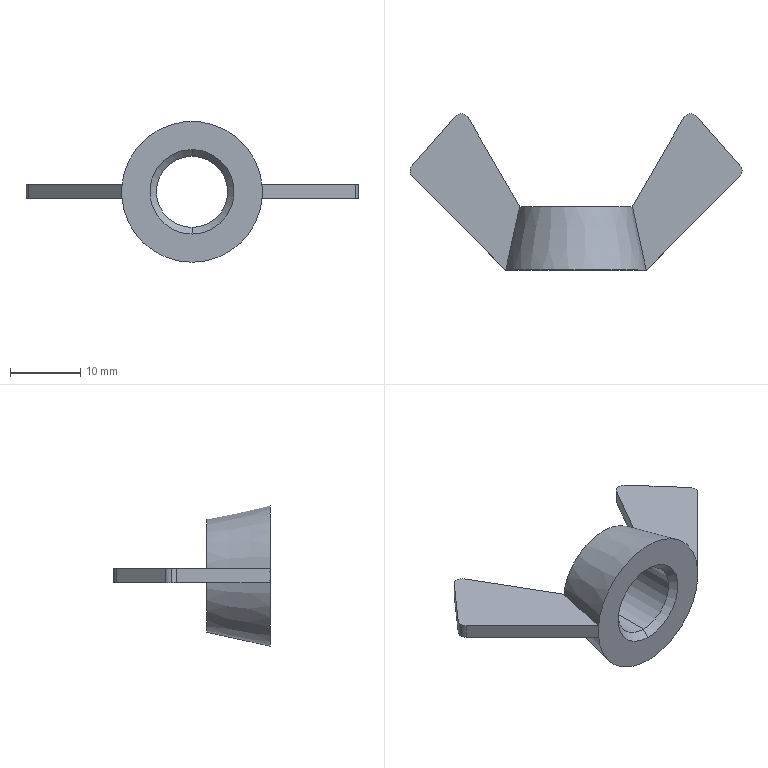Part | SolidWorks | features BaseBody 1 | 1 solid | 32 faces | box 47.146 x 22.189 x 20 mm | volume 2219 mm3 | plane 16 | cone 9 | cylinder 7 | commonest cylinder face diameters 2.3 x5 10.106 x2
STEP:
#1=CARTESIAN_POINT('',(-23.573,9.57,1.));
#2=VERTEX_POINT('',#1);
#3=CARTESIAN_POINT('',(-23.236,8.756,1.));
#4=VERTEX_POINT('',#3);
#5=CARTESIAN_POINT('',(-22.423,9.57,1.));
#6=DIRECTION('',(0.,0.,1.));
#7=DIRECTION('',(1.,0.,0.));
#8=AXIS2_PLACEMENT_3D('',#5,#6,#7);
#9=CIRCLE('',#8,1.15);
#10=EDGE_CURVE('',#2,#4,#9,.T.);
#11=ORIENTED_EDGE('',*,*,#10,.F.);
#12=CARTESIAN_POINT('',(-23.573,9.57,-1.));
#13=VERTEX_POINT('',#12);
#14=CARTESIAN_POINT('',(-23.573,9.57,1.));
#15=DIRECTION('',(0.,0.,-1.));
#16=VECTOR('',#15,1000.);
#17=LINE('',#14,#16);
#18=EDGE_CURVE('',#2,#13,#17,.T.);
#19=ORIENTED_EDGE('',*,*,#18,.T.);
#20=CARTESIAN_POINT('',(-23.236,8.756,-1.));
#21=VERTEX_POINT('',#20);
#22=CARTESIAN_POINT('',(-22.423,9.57,-1.));
#23=DIRECTION('',(0.,0.,1.));
#24=DIRECTION('',(1.,0.,0.));
#25=AXIS2_PLACEMENT_3D('',#22,#23,#24);
#26=CIRCLE('',#25,1.15);
#27=EDGE_CURVE('',#13,#21,#26,.T.);
#28=ORIENTED_EDGE('',*,*,#27,.T.);
#29=CARTESIAN_POINT('',(-23.236,8.756,1.));
#30=DIRECTION('',(0.,0.,-1.));
#31=VECTOR('',#30,1000.);
#32=LINE('',#29,#31);
#33=EDGE_CURVE('',#4,#21,#32,.T.);
#34=ORIENTED_EDGE('',*,*,#33,.F.);
#35=EDGE_LOOP('',(#11,#19,#28,#34));
#36=FACE_OUTER_BOUND('',#35,.T.);
#37=CARTESIAN_POINT('',(-22.423,9.57,1.));
#38=DIRECTION('',(0.,0.,-1.));
#39=DIRECTION('',(-1.,0.,0.));
#40=AXIS2_PLACEMENT_3D('',#37,#38,#39);
#41=CYLINDRICAL_SURFACE('',#40,1.15);
#42=ADVANCED_FACE('',(#36),#41,.T.);
#43=CARTESIAN_POINT('',(0.,3.553,5.053));
#44=VERTEX_POINT('',#43);
#45=CARTESIAN_POINT('',(0.,3.553,-5.053));
#46=VERTEX_POINT('',#45);
#47=CARTESIAN_POINT('',(0.,3.553,0.));
#48=DIRECTION('',(0.,-1.,0.));
#49=DIRECTION('',(0.,0.,-1.));
#50=AXIS2_PLACEMENT_3D('',#47,#48,#49);
#51=CIRCLE('',#50,5.053);
#52=EDGE_CURVE('',#44,#46,#51,.T.);
#53=ORIENTED_EDGE('',*,*,#52,.T.);
#54=CARTESIAN_POINT('',(0.,4.5,-6.));
#55=VERTEX_POINT('',#54);
#56=CARTESIAN_POINT('',(0.,4.5,-6.));
#57=DIRECTION('',(0.,0.7071,-0.7071));
#58=VECTOR('',#57,1000.);
#59=LINE('',#56,#58);
#60=EDGE_CURVE('',#46,#55,#59,.T.);
#61=ORIENTED_EDGE('',*,*,#60,.T.);
#62=CARTESIAN_POINT('',(0.,4.5,6.));
#63=VERTEX_POINT('',#62);
#64=CARTESIAN_POINT('',(0.,4.5,0.));
#65=DIRECTION('',(0.,-1.,0.));
#66=DIRECTION('',(0.,0.,-1.));
#67=AXIS2_PLACEMENT_3D('',#64,#65,#66);
#68=CIRCLE('',#67,6.);
#69=EDGE_CURVE('',#63,#55,#68,.T.);
#70=ORIENTED_EDGE('',*,*,#69,.F.);
#71=CARTESIAN_POINT('',(0.,4.5,6.));
#72=DIRECTION('',(0.,0.7071,0.7071));
#73=VECTOR('',#72,1000.);
#74=LINE('',#71,#73);
#75=EDGE_CURVE('',#44,#63,#74,.T.);
#76=ORIENTED_EDGE('',*,*,#75,.F.);
#77=EDGE_LOOP('',(#53,#61,#70,#76));
#78=FACE_OUTER_BOUND('',#77,.T.);
#79=CARTESIAN_POINT('',(0.,4.5,0.));
#80=DIRECTION('',(0.,1.,0.));
#81=DIRECTION('',(0.,0.,1.));
#82=AXIS2_PLACEMENT_3D('',#79,#80,#81);
#83=CONICAL_SURFACE('',#82,6.,0.7854);
#84=ADVANCED_FACE('',(#78),#83,.F.);
#85=ORIENTED_EDGE('',*,*,#52,.F.);
#86=CARTESIAN_POINT('',(0.,-3.553,5.053));
#87=VERTEX_POINT('',#86);
#88=CARTESIAN_POINT('',(0.,4.5,5.053));
#89=DIRECTION('',(0.,-1.,0.));
#90=VECTOR('',#89,1000.);
#91=LINE('',#88,#90);
#92=EDGE_CURVE('',#44,#87,#91,.T.);
#93=ORIENTED_EDGE('',*,*,#92,.T.);
#94=CARTESIAN_POINT('',(0.,-3.553,-5.053));
#95=VERTEX_POINT('',#94);
#96=CARTESIAN_POINT('',(0.,-3.553,0.));
#97=DIRECTION('',(0.,-1.,0.));
#98=DIRECTION('',(0.,0.,-1.));
#99=AXIS2_PLACEMENT_3D('',#96,#97,#98);
#100=CIRCLE('',#99,5.053);
#101=EDGE_CURVE('',#87,#95,#100,.T.);
#102=ORIENTED_EDGE('',*,*,#101,.T.);
#103=CARTESIAN_POINT('',(0.,4.5,-5.053));
#104=DIRECTION('',(0.,-1.,0.));
#105=VECTOR('',#104,1000.);
#106=LINE('',#103,#105);
#107=EDGE_CURVE('',#46,#95,#106,.T.);
#108=ORIENTED_EDGE('',*,*,#107,.F.);
#109=EDGE_LOOP('',(#85,#93,#102,#108));
#110=FACE_OUTER_BOUND('',#109,.T.);
#111=CARTESIAN_POINT('',(0.,4.5,0.));
#112=DIRECTION('',(0.,-1.,0.));
#113=DIRECTION('',(0.,0.,-1.));
#114=AXIS2_PLACEMENT_3D('',#111,#112,#113);
#115=CYLINDRICAL_SURFACE('',#114,5.053);
#116=ADVANCED_FACE('',(#110),#115,.F.);
#117=ORIENTED_EDGE('',*,*,#101,.F.);
#118=CARTESIAN_POINT('',(0.,-4.5,6.));
#119=VERTEX_POINT('',#118);
#120=CARTESIAN_POINT('',(0.,-3.553,5.053));
#121=DIRECTION('',(0.,-0.7071,0.7071));
#122=VECTOR('',#121,1000.);
#123=LINE('',#120,#122);
#124=EDGE_CURVE('',#87,#119,#123,.T.);
#125=ORIENTED_EDGE('',*,*,#124,.T.);
#126=CARTESIAN_POINT('',(0.,-4.5,-6.));
#127=VERTEX_POINT('',#126);
#128=CARTESIAN_POINT('',(0.,-4.5,0.));
#129=DIRECTION('',(0.,-1.,0.));
#130=DIRECTION('',(0.,0.,-1.));
#131=AXIS2_PLACEMENT_3D('',#128,#129,#130);
#132=CIRCLE('',#131,6.);
#133=EDGE_CURVE('',#119,#127,#132,.T.);
#134=ORIENTED_EDGE('',*,*,#133,.T.);
#135=CARTESIAN_POINT('',(0.,-3.553,-5.053));
#136=DIRECTION('',(0.,-0.7071,-0.7071));
#137=VECTOR('',#136,1000.);
#138=LINE('',#135,#137);
#139=EDGE_CURVE('',#95,#127,#138,.T.);
#140=ORIENTED_EDGE('',*,*,#139,.F.);
#141=EDGE_LOOP('',(#117,#125,#134,#140));
#142=FACE_OUTER_BOUND('',#141,.T.);
#143=CARTESIAN_POINT('',(0.,-3.553,0.));
#144=DIRECTION('',(0.,-1.,0.));
#145=DIRECTION('',(0.,0.,-1.));
#146=AXIS2_PLACEMENT_3D('',#143,#144,#145);
#147=CONICAL_SURFACE('',#146,5.053,0.7854);
#148=ADVANCED_FACE('',(#142),#147,.F.);
#149=CARTESIAN_POINT('',(-8.,4.5,0.));
#150=VERTEX_POINT('',#149);
#151=CARTESIAN_POINT('',(0.,4.5,-8.));
#152=VERTEX_POINT('',#151);
#153=CARTESIAN_POINT('',(0.,4.5,0.));
#154=DIRECTION('',(0.,-1.,0.));
#155=DIRECTION('',(0.,0.,-1.));
#156=AXIS2_PLACEMENT_3D('',#153,#154,#155);
#157=CIRCLE('',#156,8.);
#158=EDGE_CURVE('',#150,#152,#157,.T.);
#159=ORIENTED_EDGE('',*,*,#158,.T.);
#160=CARTESIAN_POINT('',(0.,-4.5,-10.));
#161=VERTEX_POINT('',#160);
#162=CARTESIAN_POINT('',(0.,4.5,-8.));
#163=DIRECTION('',(0.,-0.9762,-0.2169));
#164=VECTOR('',#163,1000.);
#165=LINE('',#162,#164);
#166=EDGE_CURVE('',#152,#161,#165,.T.);
#167=ORIENTED_EDGE('',*,*,#166,.T.);
#168=CARTESIAN_POINT('',(-9.98,-4.5,-0.6321));
#169=VERTEX_POINT('',#168);
#170=CARTESIAN_POINT('',(0.,-4.5,0.));
#171=DIRECTION('',(0.,-1.,0.));
#172=DIRECTION('',(0.,0.,-1.));
#173=AXIS2_PLACEMENT_3D('',#170,#171,#172);
#174=CIRCLE('',#173,10.);
#175=EDGE_CURVE('',#169,#161,#174,.T.);
#176=ORIENTED_EDGE('',*,*,#175,.F.);
#177=CARTESIAN_POINT('',(-8.,4.5,0.));
#178=CARTESIAN_POINT('',(-8.,4.5,-0.01244));
#179=CARTESIAN_POINT('',(-8.003,4.489,-0.02117));
#180=CARTESIAN_POINT('',(-8.007,4.468,-0.03411));
#181=CARTESIAN_POINT('',(-8.009,4.458,-0.03905));
#182=CARTESIAN_POINT('',(-8.017,4.425,-0.0525));
#183=CARTESIAN_POINT('',(-8.022,4.402,-0.0594));
#184=CARTESIAN_POINT('',(-8.037,4.334,-0.07803));
#185=CARTESIAN_POINT('',(-8.047,4.288,-0.08757));
#186=CARTESIAN_POINT('',(-8.077,4.149,-0.1136));
#187=CARTESIAN_POINT('',(-8.098,4.055,-0.1271));
#188=CARTESIAN_POINT('',(-8.16,3.775,-0.1639));
#189=CARTESIAN_POINT('',(-8.201,3.587,-0.1831));
#190=CARTESIAN_POINT('',(-8.325,3.025,-0.236));
#191=CARTESIAN_POINT('',(-8.407,2.649,-0.264));
#192=CARTESIAN_POINT('',(-8.655,1.521,-0.3417));
#193=CARTESIAN_POINT('',(-8.821,0.7688,-0.3839));
#194=CARTESIAN_POINT('',(-9.318,-1.489,-0.5022));
#195=CARTESIAN_POINT('',(-9.649,-2.994,-0.5687));
#196=CARTESIAN_POINT('',(-9.98,-4.5,-0.6321));
#197=B_SPLINE_CURVE_WITH_KNOTS('',3,(#177,#178,#179,#180,#181,#182,#183,#184,#185,#186,#187,#188,#189,#190,#191,#192,#193,#194,#195,#196),.UNSPECIFIED.,.F.,.F.,(4,2,2,2,2,2,2,2,2,4),(0.,0.00003674,0.00007347,0.0001469,0.0002939,0.0005878,0.001176,0.002351,0.004702,0.009405),.UNSPECIFIED.);
#198=EDGE_CURVE('',#150,#169,#197,.T.);
#199=ORIENTED_EDGE('',*,*,#198,.F.);
#200=EDGE_LOOP('',(#159,#167,#176,#199));
#201=FACE_OUTER_BOUND('',#200,.T.);
#202=CARTESIAN_POINT('',(0.,4.5,0.));
#203=DIRECTION('',(0.,-1.,0.));
#204=DIRECTION('',(0.,0.,-1.));
#205=AXIS2_PLACEMENT_3D('',#202,#203,#204);
#206=CONICAL_SURFACE('',#205,8.,0.2187);
#207=ADVANCED_FACE('',(#201),#206,.T.);
#208=CARTESIAN_POINT('',(15.283,17.114,-1.));
#209=VERTEX_POINT('',#208);
#210=CARTESIAN_POINT('',(8.,4.5,-1.));
#211=VERTEX_POINT('',#210);
#212=CARTESIAN_POINT('',(15.283,17.114,-1.));
#213=DIRECTION('',(-0.5,-0.866,0.));
#214=VECTOR('',#213,1000.);
#215=LINE('',#212,#214);
#216=EDGE_CURVE('',#209,#211,#215,.T.);
#217=ORIENTED_EDGE('',*,*,#216,.F.);
#218=CARTESIAN_POINT('',(17.141,17.3,-1.));
#219=VERTEX_POINT('',#218);
#220=CARTESIAN_POINT('',(16.279,16.539,-1.));
#221=DIRECTION('',(0.,0.,1.));
#222=DIRECTION('',(1.,0.,0.));
#223=AXIS2_PLACEMENT_3D('',#220,#221,#222);
#224=CIRCLE('',#223,1.15);
#225=EDGE_CURVE('',#219,#209,#224,.T.);
#226=ORIENTED_EDGE('',*,*,#225,.F.);
#227=CARTESIAN_POINT('',(23.286,10.33,-1.));
#228=VERTEX_POINT('',#227);
#229=CARTESIAN_POINT('',(23.286,10.33,-1.));
#230=DIRECTION('',(-0.6613,0.7501,0.));
#231=VECTOR('',#230,1000.);
#232=LINE('',#229,#231);
#233=EDGE_CURVE('',#228,#219,#232,.T.);
#234=ORIENTED_EDGE('',*,*,#233,.F.);
#235=CARTESIAN_POINT('',(23.236,8.756,-1.));
#236=VERTEX_POINT('',#235);
#237=CARTESIAN_POINT('',(22.423,9.57,-1.));
#238=DIRECTION('',(0.,0.,1.));
#239=DIRECTION('',(1.,0.,0.));
#240=AXIS2_PLACEMENT_3D('',#237,#238,#239);
#241=CIRCLE('',#240,1.15);
#242=EDGE_CURVE('',#236,#228,#241,.T.);
#243=ORIENTED_EDGE('',*,*,#242,.F.);
#244=CARTESIAN_POINT('',(9.98,-4.5,-1.));
#245=VERTEX_POINT('',#244);
#246=CARTESIAN_POINT('',(9.98,-4.5,-1.));
#247=DIRECTION('',(0.7071,0.7071,0.));
#248=VECTOR('',#247,1000.);
#249=LINE('',#246,#248);
#250=EDGE_CURVE('',#245,#236,#249,.T.);
#251=ORIENTED_EDGE('',*,*,#250,.F.);
#252=CARTESIAN_POINT('',(8.,4.5,-1.));
#253=DIRECTION('',(0.2149,-0.9766,0.));
#254=VECTOR('',#253,1000.);
#255=LINE('',#252,#254);
#256=EDGE_CURVE('',#211,#245,#255,.T.);
#257=ORIENTED_EDGE('',*,*,#256,.F.);
#258=EDGE_LOOP('',(#217,#226,#234,#243,#251,#257));
#259=FACE_OUTER_BOUND('',#258,.T.);
#260=CARTESIAN_POINT('',(22.423,9.57,-1.));
#261=DIRECTION('',(0.,0.,1.));
#262=DIRECTION('',(1.,0.,0.));
#263=AXIS2_PLACEMENT_3D('',#260,#261,#262);
#264=PLANE('',#263);
#265=ADVANCED_FACE('',(#259),#264,.F.);
#266=CARTESIAN_POINT('',(15.283,17.114,1.));
#267=VERTEX_POINT('',#266);
#268=CARTESIAN_POINT('',(8.,4.5,1.));
#269=VERTEX_POINT('',#268);
#270=CARTESIAN_POINT('',(15.283,17.114,1.));
#271=DIRECTION('',(-0.5,-0.866,0.));
#272=VECTOR('',#271,1000.);
#273=LINE('',#270,#272);
#274=EDGE_CURVE('',#267,#269,#273,.T.);
#275=ORIENTED_EDGE('',*,*,#274,.T.);
#276=CARTESIAN_POINT('',(9.98,-4.5,1.));
#277=VERTEX_POINT('',#276);
#278=CARTESIAN_POINT('',(8.,4.5,1.));
#279=DIRECTION('',(0.2149,-0.9766,0.));
#280=VECTOR('',#279,1000.);
#281=LINE('',#278,#280);
#282=EDGE_CURVE('',#269,#277,#281,.T.);
#283=ORIENTED_EDGE('',*,*,#282,.T.);
#284=CARTESIAN_POINT('',(23.236,8.756,1.));
#285=VERTEX_POINT('',#284);
#286=CARTESIAN_POINT('',(9.98,-4.5,1.));
#287=DIRECTION('',(0.7071,0.7071,0.));
#288=VECTOR('',#287,1000.);
#289=LINE('',#286,#288);
#290=EDGE_CURVE('',#277,#285,#289,.T.);
#291=ORIENTED_EDGE('',*,*,#290,.T.);
#292=CARTESIAN_POINT('',(23.286,10.33,1.));
#293=VERTEX_POINT('',#292);
#294=CARTESIAN_POINT('',(22.423,9.57,1.));
#295=DIRECTION('',(0.,0.,1.));
#296=DIRECTION('',(1.,0.,0.));
#297=AXIS2_PLACEMENT_3D('',#294,#295,#296);
#298=CIRCLE('',#297,1.15);
#299=EDGE_CURVE('',#285,#293,#298,.T.);
#300=ORIENTED_EDGE('',*,*,#299,.T.);
#301=CARTESIAN_POINT('',(17.141,17.3,1.));
#302=VERTEX_POINT('',#301);
#303=CARTESIAN_POINT('',(23.286,10.33,1.));
#304=DIRECTION('',(-0.6613,0.7501,0.));
#305=VECTOR('',#304,1000.);
#306=LINE('',#303,#305);
#307=EDGE_CURVE('',#293,#302,#306,.T.);
#308=ORIENTED_EDGE('',*,*,#307,.T.);
#309=CARTESIAN_POINT('',(16.279,16.539,1.));
#310=DIRECTION('',(0.,0.,1.));
#311=DIRECTION('',(1.,0.,0.));
#312=AXIS2_PLACEMENT_3D('',#309,#310,#311);
#313=CIRCLE('',#312,1.15);
#314=EDGE_CURVE('',#302,#267,#313,.T.);
#315=ORIENTED_EDGE('',*,*,#314,.T.);
#316=EDGE_LOOP('',(#275,#283,#291,#300,#308,#315));
#317=FACE_OUTER_BOUND('',#316,.T.);
#318=CARTESIAN_POINT('',(22.423,9.57,1.));
#319=DIRECTION('',(0.,0.,1.));
#320=DIRECTION('',(1.,0.,0.));
#321=AXIS2_PLACEMENT_3D('',#318,#319,#320);
#322=PLANE('',#321);
#323=ADVANCED_FACE('',(#317),#322,.T.);
#324=CARTESIAN_POINT('',(17.141,17.3,1.));
#325=DIRECTION('',(0.,0.,-1.));
#326=VECTOR('',#325,1000.);
#327=LINE('',#324,#326);
#328=EDGE_CURVE('',#302,#219,#327,.T.);
#329=ORIENTED_EDGE('',*,*,#328,.T.);
#330=ORIENTED_EDGE('',*,*,#225,.T.);
#331=CARTESIAN_POINT('',(15.283,17.114,1.));
#332=DIRECTION('',(0.,0.,-1.));
#333=VECTOR('',#332,1000.);
#334=LINE('',#331,#333);
#335=EDGE_CURVE('',#267,#209,#334,.T.);
#336=ORIENTED_EDGE('',*,*,#335,.F.);
#337=ORIENTED_EDGE('',*,*,#314,.F.);
#338=EDGE_LOOP('',(#329,#330,#336,#337));
#339=FACE_OUTER_BOUND('',#338,.T.);
#340=CARTESIAN_POINT('',(16.279,16.539,1.));
#341=DIRECTION('',(0.,0.,-1.));
#342=DIRECTION('',(-1.,0.,0.));
#343=AXIS2_PLACEMENT_3D('',#340,#341,#342);
#344=CYLINDRICAL_SURFACE('',#343,1.15);
#345=ADVANCED_FACE('',(#339),#344,.T.);
#346=CARTESIAN_POINT('',(23.286,10.33,1.));
#347=DIRECTION('',(0.,0.,-1.));
#348=VECTOR('',#347,1000.);
#349=LINE('',#346,#348);
#350=EDGE_CURVE('',#293,#228,#349,.T.);
#351=ORIENTED_EDGE('',*,*,#350,.T.);
#352=ORIENTED_EDGE('',*,*,#233,.T.);
#353=ORIENTED_EDGE('',*,*,#328,.F.);
#354=ORIENTED_EDGE('',*,*,#307,.F.);
#355=EDGE_LOOP('',(#351,#352,#353,#354));
#356=FACE_OUTER_BOUND('',#355,.T.);
#357=CARTESIAN_POINT('',(23.286,10.33,1.));
#358=DIRECTION('',(-0.7501,-0.6613,0.));
#359=DIRECTION('',(-0.6613,0.7501,0.));
#360=AXIS2_PLACEMENT_3D('',#357,#358,#359);
#361=PLANE('',#360);
#362=ADVANCED_FACE('',(#356),#361,.F.);
#363=CARTESIAN_POINT('',(23.236,8.756,1.));
#364=DIRECTION('',(0.,0.,-1.));
#365=VECTOR('',#364,1000.);
#366=LINE('',#363,#365);
#367=EDGE_CURVE('',#285,#236,#366,.T.);
#368=ORIENTED_EDGE('',*,*,#367,.T.);
#369=ORIENTED_EDGE('',*,*,#242,.T.);
#370=ORIENTED_EDGE('',*,*,#350,.F.);
#371=ORIENTED_EDGE('',*,*,#299,.F.);
#372=EDGE_LOOP('',(#368,#369,#370,#371));
#373=FACE_OUTER_BOUND('',#372,.T.);
#374=CARTESIAN_POINT('',(22.423,9.57,1.));
#375=DIRECTION('',(0.,0.,-1.));
#376=DIRECTION('',(-1.,0.,0.));
#377=AXIS2_PLACEMENT_3D('',#374,#375,#376);
#378=CYLINDRICAL_SURFACE('',#377,1.15);
#379=ADVANCED_FACE('',(#373),#378,.T.);
#380=ORIENTED_EDGE('',*,*,#335,.T.);
#381=ORIENTED_EDGE('',*,*,#216,.T.);
#382=CARTESIAN_POINT('',(8.,4.5,0.));
#383=VERTEX_POINT('',#382);
#384=CARTESIAN_POINT('',(8.,4.5,1.));
#385=DIRECTION('',(0.,0.,-1.));
#386=VECTOR('',#385,1000.);
#387=LINE('',#384,#386);
#388=EDGE_CURVE('',#383,#211,#387,.T.);
#389=ORIENTED_EDGE('',*,*,#388,.F.);
#390=CARTESIAN_POINT('',(8.,4.5,1.));
#391=DIRECTION('',(0.,0.,-1.));
#392=VECTOR('',#391,1000.);
#393=LINE('',#390,#392);
#394=EDGE_CURVE('',#269,#383,#393,.T.);
#395=ORIENTED_EDGE('',*,*,#394,.F.);
#396=ORIENTED_EDGE('',*,*,#274,.F.);
#397=EDGE_LOOP('',(#380,#381,#389,#395,#396));
#398=FACE_OUTER_BOUND('',#397,.T.);
#399=CARTESIAN_POINT('',(15.283,17.114,1.));
#400=DIRECTION('',(0.866,-0.5,0.));
#401=DIRECTION('',(0.,0.,-1.));
#402=AXIS2_PLACEMENT_3D('',#399,#400,#401);
#403=PLANE('',#402);
#404=ADVANCED_FACE('',(#398),#403,.F.);
#405=ORIENTED_EDGE('',*,*,#394,.T.);
#406=CARTESIAN_POINT('',(9.98,-4.5,0.6321));
#407=VERTEX_POINT('',#406);
#408=CARTESIAN_POINT('',(8.,4.5,0.));
#409=CARTESIAN_POINT('',(8.,4.5,0.01244));
#410=CARTESIAN_POINT('',(8.003,4.489,0.02117));
#411=CARTESIAN_POINT('',(8.007,4.468,0.03411));
#412=CARTESIAN_POINT('',(8.009,4.458,0.03905));
#413=CARTESIAN_POINT('',(8.017,4.425,0.0525));
#414=CARTESIAN_POINT('',(8.022,4.402,0.0594));
#415=CARTESIAN_POINT('',(8.037,4.334,0.07803));
#416=CARTESIAN_POINT('',(8.047,4.288,0.08757));
#417=CARTESIAN_POINT('',(8.077,4.149,0.1136));
#418=CARTESIAN_POINT('',(8.098,4.055,0.1271));
#419=CARTESIAN_POINT('',(8.16,3.775,0.1639));
#420=CARTESIAN_POINT('',(8.201,3.587,0.1831));
#421=CARTESIAN_POINT('',(8.325,3.025,0.236));
#422=CARTESIAN_POINT('',(8.407,2.649,0.264));
#423=CARTESIAN_POINT('',(8.655,1.521,0.3417));
#424=CARTESIAN_POINT('',(8.821,0.7688,0.3839));
#425=CARTESIAN_POINT('',(9.318,-1.489,0.5022));
#426=CARTESIAN_POINT('',(9.649,-2.994,0.5687));
#427=CARTESIAN_POINT('',(9.98,-4.5,0.6321));
#428=B_SPLINE_CURVE_WITH_KNOTS('',3,(#408,#409,#410,#411,#412,#413,#414,#415,#416,#417,#418,#419,#420,#421,#422,#423,#424,#425,#426,#427),.UNSPECIFIED.,.F.,.F.,(4,2,2,2,2,2,2,2,2,4),(0.,0.00003674,0.00007347,0.0001469,0.0002939,0.0005878,0.001176,0.002351,0.004702,0.009405),.UNSPECIFIED.);
#429=EDGE_CURVE('',#383,#407,#428,.T.);
#430=ORIENTED_EDGE('',*,*,#429,.T.);
#431=CARTESIAN_POINT('',(9.98,-4.5,1.));
#432=DIRECTION('',(0.,0.,-1.));
#433=VECTOR('',#432,1000.);
#434=LINE('',#431,#433);
#435=EDGE_CURVE('',#277,#407,#434,.T.);
#436=ORIENTED_EDGE('',*,*,#435,.F.);
#437=ORIENTED_EDGE('',*,*,#282,.F.);
#438=EDGE_LOOP('',(#405,#430,#436,#437));
#439=FACE_OUTER_BOUND('',#438,.T.);
#440=CARTESIAN_POINT('',(8.,4.5,1.));
#441=DIRECTION('',(0.9766,0.2149,0.));
#442=DIRECTION('',(0.,0.,-1.));
#443=AXIS2_PLACEMENT_3D('',#440,#441,#442);
#444=PLANE('',#443);
#445=ADVANCED_FACE('',(#439),#444,.F.);
#446=CARTESIAN_POINT('',(9.98,-4.5,-0.6321));
#447=VERTEX_POINT('',#446);
#448=CARTESIAN_POINT('',(9.98,-4.5,1.));
#449=DIRECTION('',(0.,0.,-1.));
#450=VECTOR('',#449,1000.);
#451=LINE('',#448,#450);
#452=EDGE_CURVE('',#447,#245,#451,.T.);
#453=ORIENTED_EDGE('',*,*,#452,.F.);
#454=CARTESIAN_POINT('',(9.98,-4.5,-0.6321));
#455=CARTESIAN_POINT('',(9.761,-3.505,-0.5902));
#456=CARTESIAN_POINT('',(9.542,-2.51,-0.5466));
#457=CARTESIAN_POINT('',(9.323,-1.515,-0.4994));
#458=CARTESIAN_POINT('',(9.177,-0.8499,-0.4679));
#459=CARTESIAN_POINT('',(9.031,-0.1844,-0.4347));
#460=CARTESIAN_POINT('',(8.884,0.4808,-0.3985));
#461=CARTESIAN_POINT('',(8.786,0.9259,-0.3742));
#462=CARTESIAN_POINT('',(8.688,1.371,-0.3485));
#463=CARTESIAN_POINT('',(8.591,1.816,-0.3202));
#464=CARTESIAN_POINT('',(8.525,2.114,-0.3012));
#465=CARTESIAN_POINT('',(8.46,2.411,-0.281));
#466=CARTESIAN_POINT('',(8.394,2.709,-0.2585));
#467=CARTESIAN_POINT('',(8.35,2.908,-0.2435));
#468=CARTESIAN_POINT('',(8.306,3.107,-0.2274));
#469=CARTESIAN_POINT('',(8.263,3.306,-0.2094));
#470=CARTESIAN_POINT('',(8.233,3.439,-0.1974));
#471=CARTESIAN_POINT('',(8.204,3.572,-0.1845));
#472=CARTESIAN_POINT('',(8.175,3.705,-0.1699));
#473=CARTESIAN_POINT('',(8.155,3.794,-0.1602));
#474=CARTESIAN_POINT('',(8.136,3.884,-0.1497));
#475=CARTESIAN_POINT('',(8.116,3.972,-0.138));
#476=CARTESIAN_POINT('',(8.103,4.032,-0.13));
#477=CARTESIAN_POINT('',(8.09,4.092,-0.1215));
#478=CARTESIAN_POINT('',(8.077,4.151,-0.1119));
#479=CARTESIAN_POINT('',(8.068,4.191,-0.1055));
#480=CARTESIAN_POINT('',(8.059,4.231,-0.0985));
#481=CARTESIAN_POINT('',(8.05,4.27,-0.09062));
#482=CARTESIAN_POINT('',(8.045,4.297,-0.08531));
#483=CARTESIAN_POINT('',(8.039,4.324,-0.07959));
#484=CARTESIAN_POINT('',(8.033,4.35,-0.0731));
#485=CARTESIAN_POINT('',(8.029,4.368,-0.06871));
#486=CARTESIAN_POINT('',(8.025,4.386,-0.06397));
#487=CARTESIAN_POINT('',(8.021,4.404,-0.05859));
#488=CARTESIAN_POINT('',(8.019,4.416,-0.05493));
#489=CARTESIAN_POINT('',(8.016,4.428,-0.05098));
#490=CARTESIAN_POINT('',(8.013,4.439,-0.04648));
#491=CARTESIAN_POINT('',(8.012,4.447,-0.0434));
#492=CARTESIAN_POINT('',(8.01,4.455,-0.04006));
#493=CARTESIAN_POINT('',(8.008,4.463,-0.03626));
#494=CARTESIAN_POINT('',(8.007,4.47,-0.03271));
#495=CARTESIAN_POINT('',(8.005,4.477,-0.02876));
#496=CARTESIAN_POINT('',(8.004,4.484,-0.02393));
#497=CARTESIAN_POINT('',(8.003,4.487,-0.02147));
#498=CARTESIAN_POINT('',(8.002,4.49,-0.01876));
#499=CARTESIAN_POINT('',(8.002,4.493,-0.01566));
#500=CARTESIAN_POINT('',(8.001,4.495,-0.01339));
#501=CARTESIAN_POINT('',(8.001,4.497,-0.01086));
#502=CARTESIAN_POINT('',(8.,4.498,-0.008086));
#503=CARTESIAN_POINT('',(8.,4.499,-0.006137));
#504=CARTESIAN_POINT('',(8.,4.5,-0.004024));
#505=CARTESIAN_POINT('',(8.,4.5,-0.001887));
#506=CARTESIAN_POINT('',(8.,4.5,-0.001261));
#507=CARTESIAN_POINT('',(8.,4.5,-0.0006299));
#508=CARTESIAN_POINT('',(8.,4.5,0.));
#509=B_SPLINE_CURVE_WITH_KNOTS('',3,(#454,#455,#456,#457,#458,#459,#460,#461,#462,#463,#464,#465,#466,#467,#468,#469,#470,#471,#472,#473,#474,#475,#476,#477,#478,#479,#480,#481,#482,#483,#484,#485,#486,#487,#488,#489,#490,#491,#492,#493,#494,#495,#496,#497,#498,#499,#500,#501,#502,#503,#504,#505,#506,#507,#508),.UNSPECIFIED.,.F.,.F.,(4,3,3,3,3,3,3,3,3,3,3,3,3,3,3,3,3,3,4),(0.,0.003059,0.005105,0.006475,0.007391,0.008004,0.008415,0.00869,0.008875,0.008999,0.009083,0.00914,0.009178,0.009204,0.009229,0.009242,0.009251,0.009257,0.009259),.UNSPECIFIED.);
#510=EDGE_CURVE('',#447,#383,#509,.T.);
#511=ORIENTED_EDGE('',*,*,#510,.T.);
#512=ORIENTED_EDGE('',*,*,#388,.T.);
#513=ORIENTED_EDGE('',*,*,#256,.T.);
#514=EDGE_LOOP('',(#453,#511,#512,#513));
#515=FACE_OUTER_BOUND('',#514,.T.);
#516=CARTESIAN_POINT('',(8.,4.5,1.));
#517=DIRECTION('',(0.9766,0.2149,0.));
#518=DIRECTION('',(0.,0.,-1.));
#519=AXIS2_PLACEMENT_3D('',#516,#517,#518);
#520=PLANE('',#519);
#521=ADVANCED_FACE('',(#515),#520,.F.);
#522=ORIENTED_EDGE('',*,*,#435,.T.);
#523=CARTESIAN_POINT('',(9.98,-4.5,0.6321));
#524=CARTESIAN_POINT('',(10.002,-4.478,0.2109));
#525=CARTESIAN_POINT('',(10.002,-4.478,-0.2109));
#526=CARTESIAN_POINT('',(9.98,-4.5,-0.6321));
#527=(BOUNDED_CURVE()B_SPLINE_CURVE(3,(#523,#524,#525,#526),.UNSPECIFIED.,.F.,.F.)B_SPLINE_CURVE_WITH_KNOTS((4,4),(3.091,3.192),.UNSPECIFIED.)CURVE()GEOMETRIC_REPRESENTATION_ITEM()RATIONAL_B_SPLINE_CURVE((1.,0.9992,0.9992,1.))REPRESENTATION_ITEM(''));
#528=EDGE_CURVE('',#407,#447,#527,.T.);
#529=ORIENTED_EDGE('',*,*,#528,.T.);
#530=ORIENTED_EDGE('',*,*,#452,.T.);
#531=ORIENTED_EDGE('',*,*,#250,.T.);
#532=ORIENTED_EDGE('',*,*,#367,.F.);
#533=ORIENTED_EDGE('',*,*,#290,.F.);
#534=EDGE_LOOP('',(#522,#529,#530,#531,#532,#533));
#535=FACE_OUTER_BOUND('',#534,.T.);
#536=CARTESIAN_POINT('',(9.98,-4.5,1.));
#537=DIRECTION('',(-0.7071,0.7071,0.));
#538=DIRECTION('',(0.,0.,1.));
#539=AXIS2_PLACEMENT_3D('',#536,#537,#538);
#540=PLANE('',#539);
#541=ADVANCED_FACE('',(#535),#540,.F.);
#542=CARTESIAN_POINT('',(-23.286,10.33,-1.));
#543=VERTEX_POINT('',#542);
#544=CARTESIAN_POINT('',(-22.423,9.57,-1.));
#545=DIRECTION('',(0.,0.,1.));
#546=DIRECTION('',(1.,0.,0.));
#547=AXIS2_PLACEMENT_3D('',#544,#545,#546);
#548=CIRCLE('',#547,1.15);
#549=EDGE_CURVE('',#543,#13,#548,.T.);
#550=ORIENTED_EDGE('',*,*,#549,.F.);
#551=CARTESIAN_POINT('',(-17.141,17.3,-1.));
#552=VERTEX_POINT('',#551);
#553=CARTESIAN_POINT('',(-17.141,17.3,-1.));
#554=DIRECTION('',(-0.6613,-0.7501,0.));
#555=VECTOR('',#554,1000.);
#556=LINE('',#553,#555);
#557=EDGE_CURVE('',#552,#543,#556,.T.);
#558=ORIENTED_EDGE('',*,*,#557,.F.);
#559=CARTESIAN_POINT('',(-15.283,17.114,-1.));
#560=VERTEX_POINT('',#559);
#561=CARTESIAN_POINT('',(-16.279,16.539,-1.));
#562=DIRECTION('',(0.,0.,1.));
#563=DIRECTION('',(1.,0.,0.));
#564=AXIS2_PLACEMENT_3D('',#561,#562,#563);
#565=CIRCLE('',#564,1.15);
#566=EDGE_CURVE('',#560,#552,#565,.T.);
#567=ORIENTED_EDGE('',*,*,#566,.F.);
#568=CARTESIAN_POINT('',(-8.,4.5,-1.));
#569=VERTEX_POINT('',#568);
#570=CARTESIAN_POINT('',(-8.,4.5,-1.));
#571=DIRECTION('',(-0.5,0.866,0.));
#572=VECTOR('',#571,1000.);
#573=LINE('',#570,#572);
#574=EDGE_CURVE('',#569,#560,#573,.T.);
#575=ORIENTED_EDGE('',*,*,#574,.F.);
#576=CARTESIAN_POINT('',(-9.98,-4.5,-1.));
#577=VERTEX_POINT('',#576);
#578=CARTESIAN_POINT('',(-9.98,-4.5,-1.));
#579=DIRECTION('',(0.2149,0.9766,0.));
#580=VECTOR('',#579,1000.);
#581=LINE('',#578,#580);
#582=EDGE_CURVE('',#577,#569,#581,.T.);
#583=ORIENTED_EDGE('',*,*,#582,.F.);
#584=CARTESIAN_POINT('',(-23.236,8.756,-1.));
#585=DIRECTION('',(0.7071,-0.7071,0.));
#586=VECTOR('',#585,1000.);
#587=LINE('',#584,#586);
#588=EDGE_CURVE('',#21,#577,#587,.T.);
#589=ORIENTED_EDGE('',*,*,#588,.F.);
#590=ORIENTED_EDGE('',*,*,#27,.F.);
#591=EDGE_LOOP('',(#550,#558,#567,#575,#583,#589,#590));
#592=FACE_OUTER_BOUND('',#591,.T.);
#593=CARTESIAN_POINT('',(-22.423,9.57,-1.));
#594=DIRECTION('',(0.,0.,1.));
#595=DIRECTION('',(1.,0.,0.));
#596=AXIS2_PLACEMENT_3D('',#593,#594,#595);
#597=PLANE('',#596);
#598=ADVANCED_FACE('',(#592),#597,.F.);
#599=CARTESIAN_POINT('',(-17.141,17.3,1.));
#600=VERTEX_POINT('',#599);
#601=CARTESIAN_POINT('',(-23.286,10.33,1.));
#602=VERTEX_POINT('',#601);
#603=CARTESIAN_POINT('',(-17.141,17.3,1.));
#604=DIRECTION('',(-0.6613,-0.7501,0.));
#605=VECTOR('',#604,1000.);
#606=LINE('',#603,#605);
#607=EDGE_CURVE('',#600,#602,#606,.T.);
#608=ORIENTED_EDGE('',*,*,#607,.T.);
#609=CARTESIAN_POINT('',(-22.423,9.57,1.));
#610=DIRECTION('',(0.,0.,1.));
#611=DIRECTION('',(1.,0.,0.));
#612=AXIS2_PLACEMENT_3D('',#609,#610,#611);
#613=CIRCLE('',#612,1.15);
#614=EDGE_CURVE('',#602,#2,#613,.T.);
#615=ORIENTED_EDGE('',*,*,#614,.T.);
#616=ORIENTED_EDGE('',*,*,#10,.T.);
#617=CARTESIAN_POINT('',(-9.98,-4.5,1.));
#618=VERTEX_POINT('',#617);
#619=CARTESIAN_POINT('',(-23.236,8.756,1.));
#620=DIRECTION('',(0.7071,-0.7071,0.));
#621=VECTOR('',#620,1000.);
#622=LINE('',#619,#621);
#623=EDGE_CURVE('',#4,#618,#622,.T.);
#624=ORIENTED_EDGE('',*,*,#623,.T.);
#625=CARTESIAN_POINT('',(-8.,4.5,1.));
#626=VERTEX_POINT('',#625);
#627=CARTESIAN_POINT('',(-9.98,-4.5,1.));
#628=DIRECTION('',(0.2149,0.9766,0.));
#629=VECTOR('',#628,1000.);
#630=LINE('',#627,#629);
#631=EDGE_CURVE('',#618,#626,#630,.T.);
#632=ORIENTED_EDGE('',*,*,#631,.T.);
#633=CARTESIAN_POINT('',(-15.283,17.114,1.));
#634=VERTEX_POINT('',#633);
#635=CARTESIAN_POINT('',(-8.,4.5,1.));
#636=DIRECTION('',(-0.5,0.866,0.));
#637=VECTOR('',#636,1000.);
#638=LINE('',#635,#637);
#639=EDGE_CURVE('',#626,#634,#638,.T.);
#640=ORIENTED_EDGE('',*,*,#639,.T.);
#641=CARTESIAN_POINT('',(-16.279,16.539,1.));
#642=DIRECTION('',(0.,0.,1.));
#643=DIRECTION('',(1.,0.,0.));
#644=AXIS2_PLACEMENT_3D('',#641,#642,#643);
#645=CIRCLE('',#644,1.15);
#646=EDGE_CURVE('',#634,#600,#645,.T.);
#647=ORIENTED_EDGE('',*,*,#646,.T.);
#648=EDGE_LOOP('',(#608,#615,#616,#624,#632,#640,#647));
#649=FACE_OUTER_BOUND('',#648,.T.);
#650=CARTESIAN_POINT('',(-22.423,9.57,1.));
#651=DIRECTION('',(0.,0.,1.));
#652=DIRECTION('',(1.,0.,0.));
#653=AXIS2_PLACEMENT_3D('',#650,#651,#652);
#654=PLANE('',#653);
#655=ADVANCED_FACE('',(#649),#654,.T.);
#656=CARTESIAN_POINT('',(-17.141,17.3,1.));
#657=DIRECTION('',(0.,0.,-1.));
#658=VECTOR('',#657,1000.);
#659=LINE('',#656,#658);
#660=EDGE_CURVE('',#600,#552,#659,.T.);
#661=ORIENTED_EDGE('',*,*,#660,.T.);
#662=ORIENTED_EDGE('',*,*,#557,.T.);
#663=CARTESIAN_POINT('',(-23.286,10.33,1.));
#664=DIRECTION('',(0.,0.,-1.));
#665=VECTOR('',#664,1000.);
#666=LINE('',#663,#665);
#667=EDGE_CURVE('',#602,#543,#666,.T.);
#668=ORIENTED_EDGE('',*,*,#667,.F.);
#669=ORIENTED_EDGE('',*,*,#607,.F.);
#670=EDGE_LOOP('',(#661,#662,#668,#669));
#671=FACE_OUTER_BOUND('',#670,.T.);
#672=CARTESIAN_POINT('',(-17.141,17.3,1.));
#673=DIRECTION('',(0.7501,-0.6613,0.));
#674=DIRECTION('',(0.,0.,-1.));
#675=AXIS2_PLACEMENT_3D('',#672,#673,#674);
#676=PLANE('',#675);
#677=ADVANCED_FACE('',(#671),#676,.F.);
#678=CARTESIAN_POINT('',(-15.283,17.114,1.));
#679=DIRECTION('',(0.,0.,-1.));
#680=VECTOR('',#679,1000.);
#681=LINE('',#678,#680);
#682=EDGE_CURVE('',#634,#560,#681,.T.);
#683=ORIENTED_EDGE('',*,*,#682,.T.);
#684=ORIENTED_EDGE('',*,*,#566,.T.);
#685=ORIENTED_EDGE('',*,*,#660,.F.);
#686=ORIENTED_EDGE('',*,*,#646,.F.);
#687=EDGE_LOOP('',(#683,#684,#685,#686));
#688=FACE_OUTER_BOUND('',#687,.T.);
#689=CARTESIAN_POINT('',(-16.279,16.539,1.));
#690=DIRECTION('',(0.,0.,-1.));
#691=DIRECTION('',(-1.,0.,0.));
#692=AXIS2_PLACEMENT_3D('',#689,#690,#691);
#693=CYLINDRICAL_SURFACE('',#692,1.15);
#694=ADVANCED_FACE('',(#688),#693,.T.);
#695=CARTESIAN_POINT('',(-8.,4.5,1.));
#696=DIRECTION('',(0.,0.,-1.));
#697=VECTOR('',#696,1000.);
#698=LINE('',#695,#697);
#699=EDGE_CURVE('',#626,#150,#698,.T.);
#700=ORIENTED_EDGE('',*,*,#699,.T.);
#701=CARTESIAN_POINT('',(-8.,4.5,1.));
#702=DIRECTION('',(0.,0.,-1.));
#703=VECTOR('',#702,1000.);
#704=LINE('',#701,#703);
#705=EDGE_CURVE('',#150,#569,#704,.T.);
#706=ORIENTED_EDGE('',*,*,#705,.T.);
#707=ORIENTED_EDGE('',*,*,#574,.T.);
#708=ORIENTED_EDGE('',*,*,#682,.F.);
#709=ORIENTED_EDGE('',*,*,#639,.F.);
#710=EDGE_LOOP('',(#700,#706,#707,#708,#709));
#711=FACE_OUTER_BOUND('',#710,.T.);
#712=CARTESIAN_POINT('',(-8.,4.5,1.));
#713=DIRECTION('',(-0.866,-0.5,0.));
#714=DIRECTION('',(-0.5,0.866,0.));
#715=AXIS2_PLACEMENT_3D('',#712,#713,#714);
#716=PLANE('',#715);
#717=ADVANCED_FACE('',(#711),#716,.F.);
#718=ORIENTED_EDGE('',*,*,#705,.F.);
#719=ORIENTED_EDGE('',*,*,#198,.T.);
#720=CARTESIAN_POINT('',(-9.98,-4.5,1.));
#721=DIRECTION('',(0.,0.,-1.));
#722=VECTOR('',#721,1000.);
#723=LINE('',#720,#722);
#724=EDGE_CURVE('',#169,#577,#723,.T.);
#725=ORIENTED_EDGE('',*,*,#724,.T.);
#726=ORIENTED_EDGE('',*,*,#582,.T.);
#727=EDGE_LOOP('',(#718,#719,#725,#726));
#728=FACE_OUTER_BOUND('',#727,.T.);
#729=CARTESIAN_POINT('',(-9.98,-4.5,1.));
#730=DIRECTION('',(-0.9766,0.2149,0.));
#731=DIRECTION('',(0.,0.,1.));
#732=AXIS2_PLACEMENT_3D('',#729,#730,#731);
#733=PLANE('',#732);
#734=ADVANCED_FACE('',(#728),#733,.F.);
#735=CARTESIAN_POINT('',(-9.98,-4.5,0.6321));
#736=VERTEX_POINT('',#735);
#737=CARTESIAN_POINT('',(-9.98,-4.5,1.));
#738=DIRECTION('',(0.,0.,-1.));
#739=VECTOR('',#738,1000.);
#740=LINE('',#737,#739);
#741=EDGE_CURVE('',#618,#736,#740,.T.);
#742=ORIENTED_EDGE('',*,*,#741,.T.);
#743=CARTESIAN_POINT('',(-9.98,-4.5,0.6321));
#744=CARTESIAN_POINT('',(-9.761,-3.505,0.5902));
#745=CARTESIAN_POINT('',(-9.542,-2.51,0.5466));
#746=CARTESIAN_POINT('',(-9.323,-1.515,0.4994));
#747=CARTESIAN_POINT('',(-9.177,-0.8499,0.4679));
#748=CARTESIAN_POINT('',(-9.031,-0.1844,0.4347));
#749=CARTESIAN_POINT('',(-8.884,0.4808,0.3985));
#750=CARTESIAN_POINT('',(-8.786,0.9259,0.3742));
#751=CARTESIAN_POINT('',(-8.688,1.371,0.3485));
#752=CARTESIAN_POINT('',(-8.591,1.816,0.3202));
#753=CARTESIAN_POINT('',(-8.525,2.114,0.3012));
#754=CARTESIAN_POINT('',(-8.46,2.411,0.281));
#755=CARTESIAN_POINT('',(-8.394,2.709,0.2585));
#756=CARTESIAN_POINT('',(-8.35,2.908,0.2435));
#757=CARTESIAN_POINT('',(-8.306,3.107,0.2274));
#758=CARTESIAN_POINT('',(-8.263,3.306,0.2094));
#759=CARTESIAN_POINT('',(-8.233,3.439,0.1974));
#760=CARTESIAN_POINT('',(-8.204,3.572,0.1845));
#761=CARTESIAN_POINT('',(-8.175,3.705,0.1699));
#762=CARTESIAN_POINT('',(-8.155,3.794,0.1602));
#763=CARTESIAN_POINT('',(-8.136,3.884,0.1497));
#764=CARTESIAN_POINT('',(-8.116,3.972,0.138));
#765=CARTESIAN_POINT('',(-8.103,4.032,0.13));
#766=CARTESIAN_POINT('',(-8.09,4.092,0.1215));
#767=CARTESIAN_POINT('',(-8.077,4.151,0.1119));
#768=CARTESIAN_POINT('',(-8.068,4.191,0.1055));
#769=CARTESIAN_POINT('',(-8.059,4.231,0.0985));
#770=CARTESIAN_POINT('',(-8.05,4.27,0.09062));
#771=CARTESIAN_POINT('',(-8.045,4.297,0.08531));
#772=CARTESIAN_POINT('',(-8.039,4.324,0.07959));
#773=CARTESIAN_POINT('',(-8.033,4.35,0.0731));
#774=CARTESIAN_POINT('',(-8.029,4.368,0.06871));
#775=CARTESIAN_POINT('',(-8.025,4.386,0.06397));
#776=CARTESIAN_POINT('',(-8.021,4.404,0.05859));
#777=CARTESIAN_POINT('',(-8.019,4.416,0.05493));
#778=CARTESIAN_POINT('',(-8.016,4.428,0.05098));
#779=CARTESIAN_POINT('',(-8.013,4.439,0.04648));
#780=CARTESIAN_POINT('',(-8.012,4.447,0.0434));
#781=CARTESIAN_POINT('',(-8.01,4.455,0.04006));
#782=CARTESIAN_POINT('',(-8.008,4.463,0.03626));
#783=CARTESIAN_POINT('',(-8.007,4.47,0.03271));
#784=CARTESIAN_POINT('',(-8.005,4.477,0.02876));
#785=CARTESIAN_POINT('',(-8.004,4.484,0.02393));
#786=CARTESIAN_POINT('',(-8.003,4.487,0.02147));
#787=CARTESIAN_POINT('',(-8.002,4.49,0.01876));
#788=CARTESIAN_POINT('',(-8.002,4.493,0.01566));
#789=CARTESIAN_POINT('',(-8.001,4.495,0.01339));
#790=CARTESIAN_POINT('',(-8.001,4.497,0.01086));
#791=CARTESIAN_POINT('',(-8.,4.498,0.008086));
#792=CARTESIAN_POINT('',(-8.,4.499,0.006137));
#793=CARTESIAN_POINT('',(-8.,4.5,0.004024));
#794=CARTESIAN_POINT('',(-8.,4.5,0.001887));
#795=CARTESIAN_POINT('',(-8.,4.5,0.001261));
#796=CARTESIAN_POINT('',(-8.,4.5,0.0006299));
#797=CARTESIAN_POINT('',(-8.,4.5,0.));
#798=B_SPLINE_CURVE_WITH_KNOTS('',3,(#743,#744,#745,#746,#747,#748,#749,#750,#751,#752,#753,#754,#755,#756,#757,#758,#759,#760,#761,#762,#763,#764,#765,#766,#767,#768,#769,#770,#771,#772,#773,#774,#775,#776,#777,#778,#779,#780,#781,#782,#783,#784,#785,#786,#787,#788,#789,#790,#791,#792,#793,#794,#795,#796,#797),.UNSPECIFIED.,.F.,.F.,(4,3,3,3,3,3,3,3,3,3,3,3,3,3,3,3,3,3,4),(0.,0.003059,0.005105,0.006475,0.007391,0.008004,0.008415,0.00869,0.008875,0.008999,0.009083,0.00914,0.009178,0.009204,0.009229,0.009242,0.009251,0.009257,0.009259),.UNSPECIFIED.);
#799=EDGE_CURVE('',#736,#150,#798,.T.);
#800=ORIENTED_EDGE('',*,*,#799,.T.);
#801=ORIENTED_EDGE('',*,*,#699,.F.);
#802=ORIENTED_EDGE('',*,*,#631,.F.);
#803=EDGE_LOOP('',(#742,#800,#801,#802));
#804=FACE_OUTER_BOUND('',#803,.T.);
#805=CARTESIAN_POINT('',(-9.98,-4.5,1.));
#806=DIRECTION('',(-0.9766,0.2149,0.));
#807=DIRECTION('',(0.,0.,1.));
#808=AXIS2_PLACEMENT_3D('',#805,#806,#807);
#809=PLANE('',#808);
#810=ADVANCED_FACE('',(#804),#809,.F.);
#811=ORIENTED_EDGE('',*,*,#724,.F.);
#812=CARTESIAN_POINT('',(-9.98,-4.5,-0.6321));
#813=CARTESIAN_POINT('',(-10.002,-4.478,-0.2109));
#814=CARTESIAN_POINT('',(-10.002,-4.478,0.2109));
#815=CARTESIAN_POINT('',(-9.98,-4.5,0.6321));
#816=(BOUNDED_CURVE()B_SPLINE_CURVE(3,(#812,#813,#814,#815),.UNSPECIFIED.,.F.,.F.)B_SPLINE_CURVE_WITH_KNOTS((4,4),(3.091,3.192),.UNSPECIFIED.)CURVE()GEOMETRIC_REPRESENTATION_ITEM()RATIONAL_B_SPLINE_CURVE((1.,0.9992,0.9992,1.))REPRESENTATION_ITEM(''));
#817=EDGE_CURVE('',#169,#736,#816,.T.);
#818=ORIENTED_EDGE('',*,*,#817,.T.);
#819=ORIENTED_EDGE('',*,*,#741,.F.);
#820=ORIENTED_EDGE('',*,*,#623,.F.);
#821=ORIENTED_EDGE('',*,*,#33,.T.);
#822=ORIENTED_EDGE('',*,*,#588,.T.);
#823=EDGE_LOOP('',(#811,#818,#819,#820,#821,#822));
#824=FACE_OUTER_BOUND('',#823,.T.);
#825=CARTESIAN_POINT('',(-23.236,8.756,1.));
#826=DIRECTION('',(0.7071,0.7071,0.));
#827=DIRECTION('',(0.,0.,-1.));
#828=AXIS2_PLACEMENT_3D('',#825,#826,#827);
#829=PLANE('',#828);
#830=ADVANCED_FACE('',(#824),#829,.F.);
#831=ORIENTED_EDGE('',*,*,#69,.T.);
#832=CARTESIAN_POINT('',(0.,4.5,0.));
#833=DIRECTION('',(0.,-1.,0.));
#834=DIRECTION('',(0.,0.,-1.));
#835=AXIS2_PLACEMENT_3D('',#832,#833,#834);
#836=CIRCLE('',#835,6.);
#837=EDGE_CURVE('',#55,#63,#836,.T.);
#838=ORIENTED_EDGE('',*,*,#837,.T.);
#839=EDGE_LOOP('',(#831,#838));
#840=FACE_BOUND('',#839,.T.);
#841=ORIENTED_EDGE('',*,*,#158,.F.);
#842=CARTESIAN_POINT('',(0.,4.5,0.));
#843=DIRECTION('',(0.,-1.,0.));
#844=DIRECTION('',(0.,0.,-1.));
#845=AXIS2_PLACEMENT_3D('',#842,#843,#844);
#846=CIRCLE('',#845,8.);
#847=EDGE_CURVE('',#383,#150,#846,.T.);
#848=ORIENTED_EDGE('',*,*,#847,.F.);
#849=CARTESIAN_POINT('',(0.,4.5,0.));
#850=DIRECTION('',(0.,-1.,0.));
#851=DIRECTION('',(0.,0.,-1.));
#852=AXIS2_PLACEMENT_3D('',#849,#850,#851);
#853=CIRCLE('',#852,8.);
#854=EDGE_CURVE('',#152,#383,#853,.T.);
#855=ORIENTED_EDGE('',*,*,#854,.F.);
#856=EDGE_LOOP('',(#841,#848,#855));
#857=FACE_OUTER_BOUND('',#856,.T.);
#858=CARTESIAN_POINT('',(-8.,4.5,0.));
#859=DIRECTION('',(0.,-1.,0.));
#860=DIRECTION('',(0.,0.,-1.));
#861=AXIS2_PLACEMENT_3D('',#858,#859,#860);
#862=PLANE('',#861);
#863=ADVANCED_FACE('',(#840,#857),#862,.F.);
#864=CARTESIAN_POINT('',(0.,-4.5,0.));
#865=DIRECTION('',(0.,-1.,0.));
#866=DIRECTION('',(0.,0.,-1.));
#867=AXIS2_PLACEMENT_3D('',#864,#865,#866);
#868=CIRCLE('',#867,6.);
#869=EDGE_CURVE('',#127,#119,#868,.T.);
#870=ORIENTED_EDGE('',*,*,#869,.F.);
#871=ORIENTED_EDGE('',*,*,#133,.F.);
#872=EDGE_LOOP('',(#870,#871));
#873=FACE_BOUND('',#872,.T.);
#874=ORIENTED_EDGE('',*,*,#175,.T.);
#875=CARTESIAN_POINT('',(0.,-4.5,0.));
#876=DIRECTION('',(0.,-1.,0.));
#877=DIRECTION('',(0.,0.,-1.));
#878=AXIS2_PLACEMENT_3D('',#875,#876,#877);
#879=CIRCLE('',#878,10.);
#880=EDGE_CURVE('',#161,#447,#879,.T.);
#881=ORIENTED_EDGE('',*,*,#880,.T.);
#882=CARTESIAN_POINT('',(0.,-4.5,0.));
#883=DIRECTION('',(0.,-1.,0.));
#884=DIRECTION('',(0.,0.,-1.));
#885=AXIS2_PLACEMENT_3D('',#882,#883,#884);
#886=CIRCLE('',#885,10.);
#887=EDGE_CURVE('',#447,#407,#886,.T.);
#888=ORIENTED_EDGE('',*,*,#887,.T.);
#889=CARTESIAN_POINT('',(0.,-4.5,0.));
#890=DIRECTION('',(0.,-1.,0.));
#891=DIRECTION('',(0.,0.,-1.));
#892=AXIS2_PLACEMENT_3D('',#889,#890,#891);
#893=CIRCLE('',#892,10.);
#894=EDGE_CURVE('',#407,#736,#893,.T.);
#895=ORIENTED_EDGE('',*,*,#894,.T.);
#896=CARTESIAN_POINT('',(0.,-4.5,0.));
#897=DIRECTION('',(0.,-1.,0.));
#898=DIRECTION('',(0.,0.,-1.));
#899=AXIS2_PLACEMENT_3D('',#896,#897,#898);
#900=CIRCLE('',#899,10.);
#901=EDGE_CURVE('',#736,#169,#900,.T.);
#902=ORIENTED_EDGE('',*,*,#901,.T.);
#903=EDGE_LOOP('',(#874,#881,#888,#895,#902));
#904=FACE_OUTER_BOUND('',#903,.T.);
#905=CARTESIAN_POINT('',(0.,-4.5,0.));
#906=DIRECTION('',(0.,1.,0.));
#907=DIRECTION('',(1.,0.,0.));
#908=AXIS2_PLACEMENT_3D('',#905,#906,#907);
#909=PLANE('',#908);
#910=ADVANCED_FACE('',(#873,#904),#909,.F.);
#911=ORIENTED_EDGE('',*,*,#817,.F.);
#912=ORIENTED_EDGE('',*,*,#901,.F.);
#913=EDGE_LOOP('',(#911,#912));
#914=FACE_OUTER_BOUND('',#913,.T.);
#915=CARTESIAN_POINT('',(0.,4.5,0.));
#916=DIRECTION('',(0.,-1.,0.));
#917=DIRECTION('',(0.,0.,-1.));
#918=AXIS2_PLACEMENT_3D('',#915,#916,#917);
#919=CONICAL_SURFACE('',#918,8.,0.2187);
#920=ADVANCED_FACE('',(#914),#919,.T.);
#921=ORIENTED_EDGE('',*,*,#528,.F.);
#922=ORIENTED_EDGE('',*,*,#887,.F.);
#923=EDGE_LOOP('',(#921,#922));
#924=FACE_OUTER_BOUND('',#923,.T.);
#925=CARTESIAN_POINT('',(0.,4.5,0.));
#926=DIRECTION('',(0.,-1.,0.));
#927=DIRECTION('',(0.,0.,-1.));
#928=AXIS2_PLACEMENT_3D('',#925,#926,#927);
#929=CONICAL_SURFACE('',#928,8.,0.2187);
#930=ADVANCED_FACE('',(#924),#929,.T.);
#931=ORIENTED_EDGE('',*,*,#429,.F.);
#932=ORIENTED_EDGE('',*,*,#847,.T.);
#933=ORIENTED_EDGE('',*,*,#799,.F.);
#934=ORIENTED_EDGE('',*,*,#894,.F.);
#935=EDGE_LOOP('',(#931,#932,#933,#934));
#936=FACE_OUTER_BOUND('',#935,.T.);
#937=CARTESIAN_POINT('',(0.,4.5,0.));
#938=DIRECTION('',(0.,-1.,0.));
#939=DIRECTION('',(0.,0.,-1.));
#940=AXIS2_PLACEMENT_3D('',#937,#938,#939);
#941=CONICAL_SURFACE('',#940,8.,0.2187);
#942=ADVANCED_FACE('',(#936),#941,.T.);
#943=ORIENTED_EDGE('',*,*,#166,.F.);
#944=ORIENTED_EDGE('',*,*,#854,.T.);
#945=ORIENTED_EDGE('',*,*,#510,.F.);
#946=ORIENTED_EDGE('',*,*,#880,.F.);
#947=EDGE_LOOP('',(#943,#944,#945,#946));
#948=FACE_OUTER_BOUND('',#947,.T.);
#949=CARTESIAN_POINT('',(0.,4.5,0.));
#950=DIRECTION('',(0.,-1.,0.));
#951=DIRECTION('',(0.,0.,-1.));
#952=AXIS2_PLACEMENT_3D('',#949,#950,#951);
#953=CONICAL_SURFACE('',#952,8.,0.2187);
#954=ADVANCED_FACE('',(#948),#953,.T.);
#955=ORIENTED_EDGE('',*,*,#124,.F.);
#956=CARTESIAN_POINT('',(0.,-3.553,0.));
#957=DIRECTION('',(0.,-1.,0.));
#958=DIRECTION('',(0.,0.,-1.));
#959=AXIS2_PLACEMENT_3D('',#956,#957,#958);
#960=CIRCLE('',#959,5.053);
#961=EDGE_CURVE('',#95,#87,#960,.T.);
#962=ORIENTED_EDGE('',*,*,#961,.F.);
#963=ORIENTED_EDGE('',*,*,#139,.T.);
#964=ORIENTED_EDGE('',*,*,#869,.T.);
#965=EDGE_LOOP('',(#955,#962,#963,#964));
#966=FACE_OUTER_BOUND('',#965,.T.);
#967=CARTESIAN_POINT('',(0.,-3.553,0.));
#968=DIRECTION('',(0.,-1.,0.));
#969=DIRECTION('',(0.,0.,-1.));
#970=AXIS2_PLACEMENT_3D('',#967,#968,#969);
#971=CONICAL_SURFACE('',#970,5.053,0.7854);
#972=ADVANCED_FACE('',(#966),#971,.F.);
#973=ORIENTED_EDGE('',*,*,#92,.F.);
#974=CARTESIAN_POINT('',(0.,3.553,0.));
#975=DIRECTION('',(0.,-1.,0.));
#976=DIRECTION('',(0.,0.,-1.));
#977=AXIS2_PLACEMENT_3D('',#974,#975,#976);
#978=CIRCLE('',#977,5.053);
#979=EDGE_CURVE('',#46,#44,#978,.T.);
#980=ORIENTED_EDGE('',*,*,#979,.F.);
#981=ORIENTED_EDGE('',*,*,#107,.T.);
#982=ORIENTED_EDGE('',*,*,#961,.T.);
#983=EDGE_LOOP('',(#973,#980,#981,#982));
#984=FACE_OUTER_BOUND('',#983,.T.);
#985=CARTESIAN_POINT('',(0.,4.5,0.));
#986=DIRECTION('',(0.,-1.,0.));
#987=DIRECTION('',(0.,0.,-1.));
#988=AXIS2_PLACEMENT_3D('',#985,#986,#987);
#989=CYLINDRICAL_SURFACE('',#988,5.053);
#990=ADVANCED_FACE('',(#984),#989,.F.);
#991=ORIENTED_EDGE('',*,*,#60,.F.);
#992=ORIENTED_EDGE('',*,*,#979,.T.);
#993=ORIENTED_EDGE('',*,*,#75,.T.);
#994=ORIENTED_EDGE('',*,*,#837,.F.);
#995=EDGE_LOOP('',(#991,#992,#993,#994));
#996=FACE_OUTER_BOUND('',#995,.T.);
#997=CARTESIAN_POINT('',(0.,4.5,0.));
#998=DIRECTION('',(0.,1.,0.));
#999=DIRECTION('',(0.,0.,1.));
#1000=AXIS2_PLACEMENT_3D('',#997,#998,#999);
#1001=CONICAL_SURFACE('',#1000,6.,0.7854);
#1002=ADVANCED_FACE('',(#996),#1001,.F.);
#1003=ORIENTED_EDGE('',*,*,#18,.F.);
#1004=ORIENTED_EDGE('',*,*,#614,.F.);
#1005=ORIENTED_EDGE('',*,*,#667,.T.);
#1006=ORIENTED_EDGE('',*,*,#549,.T.);
#1007=EDGE_LOOP('',(#1003,#1004,#1005,#1006));
#1008=FACE_OUTER_BOUND('',#1007,.T.);
#1009=CARTESIAN_POINT('',(-22.423,9.57,1.));
#1010=DIRECTION('',(0.,0.,-1.));
#1011=DIRECTION('',(-1.,0.,0.));
#1012=AXIS2_PLACEMENT_3D('',#1009,#1010,#1011);
#1013=CYLINDRICAL_SURFACE('',#1012,1.15);
#1014=ADVANCED_FACE('',(#1008),#1013,.T.);
#1015=CLOSED_SHELL('',(#42,#84,#116,#148,#207,#265,#323,#345,#362,#379,#404,#445,#521,#541,#598,#655,#677,#694,#717,#734,#810,#830,#863,#910,#920,#930,#942,#954,#972,#990,#1002,#1014));
#1016=MANIFOLD_SOLID_BREP('',#1015);
#1017=CARTESIAN_POINT('',(0.,0.,0.));
#1018=DIRECTION('',(0.,0.,1.));
#1019=DIRECTION('',(1.,0.,0.));
#1020=AXIS2_PLACEMENT_3D('',#1017,#1018,#1019);
#1021=(LENGTH_UNIT()NAMED_UNIT(*)SI_UNIT(.MILLI.,.METRE.));
#1022=UNCERTAINTY_MEASURE_WITH_UNIT(LENGTH_MEASURE(0.00001),#1021,'','');
#1023=(NAMED_UNIT(*)PLANE_ANGLE_UNIT()SI_UNIT($,.RADIAN.));
#1024=(NAMED_UNIT(*)SI_UNIT($,.STERADIAN.)SOLID_ANGLE_UNIT());
#1025=(GEOMETRIC_REPRESENTATION_CONTEXT(3)GLOBAL_UNCERTAINTY_ASSIGNED_CONTEXT((#1022))GLOBAL_UNIT_ASSIGNED_CONTEXT((#1021,#1023,#1024))REPRESENTATION_CONTEXT('',''));
#1026=ADVANCED_BREP_SHAPE_REPRESENTATION('',(#1016,#1020),#1025);